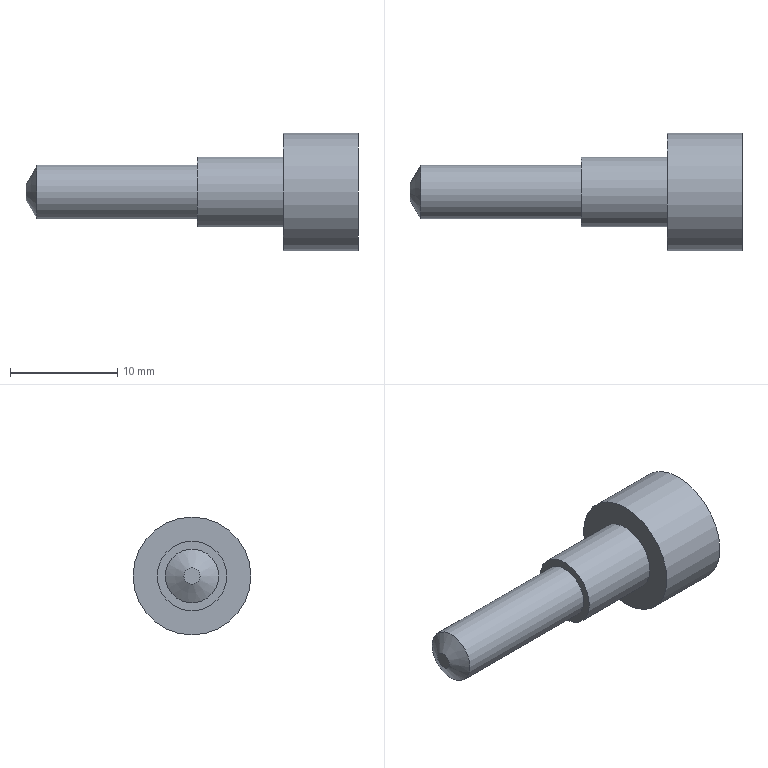Part | STEP file | solid 239 | 1 solid | 8 faces | box 31 x 11 x 11 mm | volume 1234 mm3 | plane 4 | cylinder 3 | cone 1 | commonest cylinder face diameters 5 x1 6.5 x1 11 x1